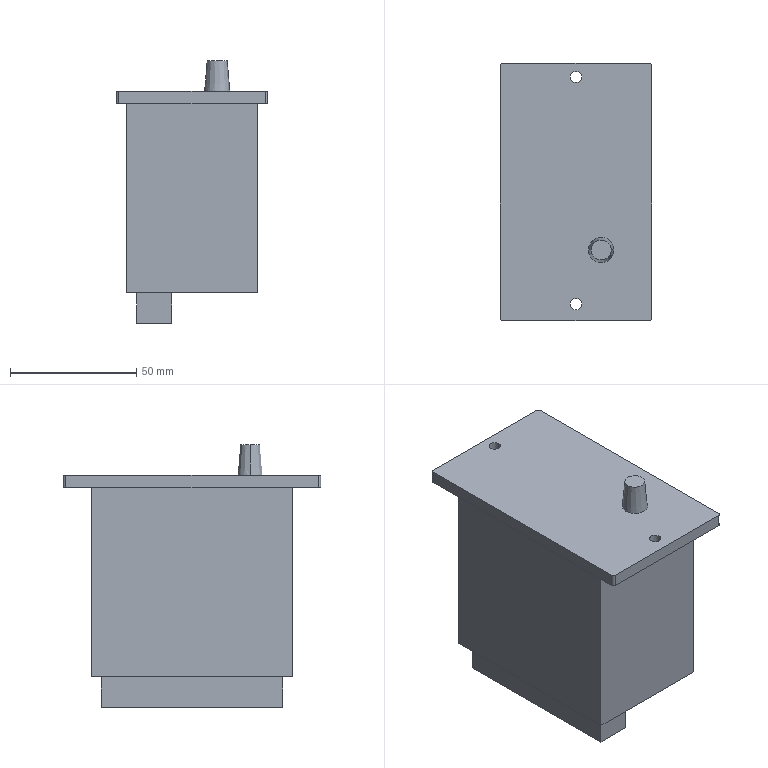Part | SolidWorks | features ICE 3, Extrusion 1, Fillet 1 | 1 solid | 27 faces | box 60 x 102 x 104 mm | volume 355291 mm3 | plane 17 | cylinder 8 | cone 2 | commonest cylinder face diameters 2 x4 4.5 x4
STEP:
#1=CARTESIAN_POINT('',(6.05,-23.,17.));
#2=VERTEX_POINT('',#1);
#3=CARTESIAN_POINT('',(13.95,-23.,17.));
#4=VERTEX_POINT('',#3);
#5=CARTESIAN_POINT('',(10.,-23.,17.));
#6=DIRECTION('',(0.,0.,1.));
#7=DIRECTION('',(1.,0.,0.));
#8=AXIS2_PLACEMENT_3D('',#5,#6,#7);
#9=CIRCLE('',#8,3.95);
#10=EDGE_CURVE('',#2,#4,#9,.T.);
#11=ORIENTED_EDGE('',*,*,#10,.F.);
#12=CARTESIAN_POINT('',(5.,-23.,5.));
#13=VERTEX_POINT('',#12);
#14=CARTESIAN_POINT('',(5.,-23.,5.));
#15=DIRECTION('',(-0.08716,0.,-0.9962));
#16=VECTOR('',#15,1000.);
#17=LINE('',#14,#16);
#18=EDGE_CURVE('',#2,#13,#17,.T.);
#19=ORIENTED_EDGE('',*,*,#18,.T.);
#20=CARTESIAN_POINT('',(15.,-23.,5.));
#21=VERTEX_POINT('',#20);
#22=CARTESIAN_POINT('',(10.,-23.,5.));
#23=DIRECTION('',(0.,0.,1.));
#24=DIRECTION('',(-1.,0.,0.));
#25=AXIS2_PLACEMENT_3D('',#22,#23,#24);
#26=CIRCLE('',#25,5.);
#27=EDGE_CURVE('',#13,#21,#26,.T.);
#28=ORIENTED_EDGE('',*,*,#27,.T.);
#29=CARTESIAN_POINT('',(15.,-23.,5.));
#30=DIRECTION('',(0.08716,0.,-0.9962));
#31=VECTOR('',#30,1000.);
#32=LINE('',#29,#31);
#33=EDGE_CURVE('',#4,#21,#32,.T.);
#34=ORIENTED_EDGE('',*,*,#33,.F.);
#35=EDGE_LOOP('',(#11,#19,#28,#34));
#36=FACE_OUTER_BOUND('',#35,.T.);
#37=CARTESIAN_POINT('',(10.,-23.,5.));
#38=DIRECTION('',(0.,0.,-1.));
#39=DIRECTION('',(1.,0.,0.));
#40=AXIS2_PLACEMENT_3D('',#37,#38,#39);
#41=CONICAL_SURFACE('',#40,5.,0.08727);
#42=ADVANCED_FACE('',(#36),#41,.T.);
#43=CARTESIAN_POINT('',(-2.25,-44.437,5.));
#44=VERTEX_POINT('',#43);
#45=CARTESIAN_POINT('',(2.25,-44.437,5.));
#46=VERTEX_POINT('',#45);
#47=CARTESIAN_POINT('',(0.,-44.437,5.));
#48=DIRECTION('',(0.,0.,1.));
#49=DIRECTION('',(1.,0.,0.));
#50=AXIS2_PLACEMENT_3D('',#47,#48,#49);
#51=CIRCLE('',#50,2.25);
#52=EDGE_CURVE('',#44,#46,#51,.T.);
#53=ORIENTED_EDGE('',*,*,#52,.T.);
#54=CARTESIAN_POINT('',(2.25,-44.437,0.));
#55=VERTEX_POINT('',#54);
#56=CARTESIAN_POINT('',(2.25,-44.437,5.));
#57=DIRECTION('',(0.,0.,-1.));
#58=VECTOR('',#57,1000.);
#59=LINE('',#56,#58);
#60=EDGE_CURVE('',#46,#55,#59,.T.);
#61=ORIENTED_EDGE('',*,*,#60,.T.);
#62=CARTESIAN_POINT('',(-2.25,-44.437,0.));
#63=VERTEX_POINT('',#62);
#64=CARTESIAN_POINT('',(0.,-44.437,0.));
#65=DIRECTION('',(0.,0.,1.));
#66=DIRECTION('',(1.,0.,0.));
#67=AXIS2_PLACEMENT_3D('',#64,#65,#66);
#68=CIRCLE('',#67,2.25);
#69=EDGE_CURVE('',#63,#55,#68,.T.);
#70=ORIENTED_EDGE('',*,*,#69,.F.);
#71=CARTESIAN_POINT('',(-2.25,-44.437,5.));
#72=DIRECTION('',(0.,0.,-1.));
#73=VECTOR('',#72,1000.);
#74=LINE('',#71,#73);
#75=EDGE_CURVE('',#44,#63,#74,.T.);
#76=ORIENTED_EDGE('',*,*,#75,.F.);
#77=EDGE_LOOP('',(#53,#61,#70,#76));
#78=FACE_OUTER_BOUND('',#77,.T.);
#79=CARTESIAN_POINT('',(0.,-44.437,5.));
#80=DIRECTION('',(0.,0.,-1.));
#81=DIRECTION('',(-1.,0.,0.));
#82=AXIS2_PLACEMENT_3D('',#79,#80,#81);
#83=CYLINDRICAL_SURFACE('',#82,2.25);
#84=ADVANCED_FACE('',(#78),#83,.F.);
#85=CARTESIAN_POINT('',(-2.25,45.563,5.));
#86=VERTEX_POINT('',#85);
#87=CARTESIAN_POINT('',(2.25,45.563,5.));
#88=VERTEX_POINT('',#87);
#89=CARTESIAN_POINT('',(0.,45.563,5.));
#90=DIRECTION('',(0.,0.,1.));
#91=DIRECTION('',(1.,0.,0.));
#92=AXIS2_PLACEMENT_3D('',#89,#90,#91);
#93=CIRCLE('',#92,2.25);
#94=EDGE_CURVE('',#86,#88,#93,.T.);
#95=ORIENTED_EDGE('',*,*,#94,.T.);
#96=CARTESIAN_POINT('',(2.25,45.563,0.));
#97=VERTEX_POINT('',#96);
#98=CARTESIAN_POINT('',(2.25,45.563,5.));
#99=DIRECTION('',(0.,0.,-1.));
#100=VECTOR('',#99,1000.);
#101=LINE('',#98,#100);
#102=EDGE_CURVE('',#88,#97,#101,.T.);
#103=ORIENTED_EDGE('',*,*,#102,.T.);
#104=CARTESIAN_POINT('',(-2.25,45.563,0.));
#105=VERTEX_POINT('',#104);
#106=CARTESIAN_POINT('',(0.,45.563,0.));
#107=DIRECTION('',(0.,0.,1.));
#108=DIRECTION('',(1.,0.,0.));
#109=AXIS2_PLACEMENT_3D('',#106,#107,#108);
#110=CIRCLE('',#109,2.25);
#111=EDGE_CURVE('',#105,#97,#110,.T.);
#112=ORIENTED_EDGE('',*,*,#111,.F.);
#113=CARTESIAN_POINT('',(-2.25,45.563,5.));
#114=DIRECTION('',(0.,0.,-1.));
#115=VECTOR('',#114,1000.);
#116=LINE('',#113,#115);
#117=EDGE_CURVE('',#86,#105,#116,.T.);
#118=ORIENTED_EDGE('',*,*,#117,.F.);
#119=EDGE_LOOP('',(#95,#103,#112,#118));
#120=FACE_OUTER_BOUND('',#119,.T.);
#121=CARTESIAN_POINT('',(0.,45.563,5.));
#122=DIRECTION('',(0.,0.,-1.));
#123=DIRECTION('',(-1.,0.,0.));
#124=AXIS2_PLACEMENT_3D('',#121,#122,#123);
#125=CYLINDRICAL_SURFACE('',#124,2.25);
#126=ADVANCED_FACE('',(#120),#125,.F.);
#127=CARTESIAN_POINT('',(-26.,-40.,-75.));
#128=VERTEX_POINT('',#127);
#129=CARTESIAN_POINT('',(-26.,40.,-75.));
#130=VERTEX_POINT('',#129);
#131=CARTESIAN_POINT('',(-26.,-40.,-75.));
#132=DIRECTION('',(0.,1.,0.));
#133=VECTOR('',#132,1000.);
#134=LINE('',#131,#133);
#135=EDGE_CURVE('',#128,#130,#134,.T.);
#136=ORIENTED_EDGE('',*,*,#135,.T.);
#137=CARTESIAN_POINT('',(26.,40.,-75.));
#138=VERTEX_POINT('',#137);
#139=CARTESIAN_POINT('',(26.,40.,-75.));
#140=DIRECTION('',(1.,0.,0.));
#141=VECTOR('',#140,1000.);
#142=LINE('',#139,#141);
#143=EDGE_CURVE('',#130,#138,#142,.T.);
#144=ORIENTED_EDGE('',*,*,#143,.T.);
#145=CARTESIAN_POINT('',(26.,-40.,-75.));
#146=VERTEX_POINT('',#145);
#147=CARTESIAN_POINT('',(26.,-40.,-75.));
#148=DIRECTION('',(0.,-1.,0.));
#149=VECTOR('',#148,1000.);
#150=LINE('',#147,#149);
#151=EDGE_CURVE('',#138,#146,#150,.T.);
#152=ORIENTED_EDGE('',*,*,#151,.T.);
#153=CARTESIAN_POINT('',(26.,-40.,-75.));
#154=DIRECTION('',(-1.,0.,0.));
#155=VECTOR('',#154,1000.);
#156=LINE('',#153,#155);
#157=EDGE_CURVE('',#146,#128,#156,.T.);
#158=ORIENTED_EDGE('',*,*,#157,.T.);
#159=EDGE_LOOP('',(#136,#144,#152,#158));
#160=FACE_OUTER_BOUND('',#159,.T.);
#161=CARTESIAN_POINT('',(-8.,36.,-75.));
#162=VERTEX_POINT('',#161);
#163=CARTESIAN_POINT('',(-8.,-36.,-75.));
#164=VERTEX_POINT('',#163);
#165=CARTESIAN_POINT('',(-8.,36.,-75.));
#166=DIRECTION('',(0.,-1.,0.));
#167=VECTOR('',#166,1000.);
#168=LINE('',#165,#167);
#169=EDGE_CURVE('',#162,#164,#168,.T.);
#170=ORIENTED_EDGE('',*,*,#169,.F.);
#171=CARTESIAN_POINT('',(-22.,36.,-75.));
#172=VERTEX_POINT('',#171);
#173=CARTESIAN_POINT('',(-8.,36.,-75.));
#174=DIRECTION('',(1.,0.,0.));
#175=VECTOR('',#174,1000.);
#176=LINE('',#173,#175);
#177=EDGE_CURVE('',#172,#162,#176,.T.);
#178=ORIENTED_EDGE('',*,*,#177,.F.);
#179=CARTESIAN_POINT('',(-22.,-36.,-75.));
#180=VERTEX_POINT('',#179);
#181=CARTESIAN_POINT('',(-22.,36.,-75.));
#182=DIRECTION('',(0.,1.,0.));
#183=VECTOR('',#182,1000.);
#184=LINE('',#181,#183);
#185=EDGE_CURVE('',#180,#172,#184,.T.);
#186=ORIENTED_EDGE('',*,*,#185,.F.);
#187=CARTESIAN_POINT('',(-8.,-36.,-75.));
#188=DIRECTION('',(-1.,0.,0.));
#189=VECTOR('',#188,1000.);
#190=LINE('',#187,#189);
#191=EDGE_CURVE('',#164,#180,#190,.T.);
#192=ORIENTED_EDGE('',*,*,#191,.F.);
#193=EDGE_LOOP('',(#170,#178,#186,#192));
#194=FACE_BOUND('',#193,.T.);
#195=CARTESIAN_POINT('',(0.,0.,-75.));
#196=DIRECTION('',(0.,0.,1.));
#197=DIRECTION('',(1.,0.,0.));
#198=AXIS2_PLACEMENT_3D('',#195,#196,#197);
#199=PLANE('',#198);
#200=ADVANCED_FACE('',(#160,#194),#199,.F.);
#201=ORIENTED_EDGE('',*,*,#52,.F.);
#202=CARTESIAN_POINT('',(0.,-44.437,5.));
#203=DIRECTION('',(0.,0.,1.));
#204=DIRECTION('',(1.,0.,0.));
#205=AXIS2_PLACEMENT_3D('',#202,#203,#204);
#206=CIRCLE('',#205,2.25);
#207=EDGE_CURVE('',#46,#44,#206,.T.);
#208=ORIENTED_EDGE('',*,*,#207,.F.);
#209=EDGE_LOOP('',(#201,#208));
#210=FACE_BOUND('',#209,.T.);
#211=CARTESIAN_POINT('',(-30.,50.,5.));
#212=VERTEX_POINT('',#211);
#213=CARTESIAN_POINT('',(-30.,-50.,5.));
#214=VERTEX_POINT('',#213);
#215=CARTESIAN_POINT('',(-30.,-51.,5.));
#216=DIRECTION('',(0.,-1.,0.));
#217=VECTOR('',#216,1000.);
#218=LINE('',#215,#217);
#219=EDGE_CURVE('',#212,#214,#218,.T.);
#220=ORIENTED_EDGE('',*,*,#219,.T.);
#221=CARTESIAN_POINT('',(-29.,-51.,5.));
#222=VERTEX_POINT('',#221);
#223=CARTESIAN_POINT('',(-29.,-50.,5.));
#224=DIRECTION('',(0.,0.,1.));
#225=DIRECTION('',(-1.,0.,0.));
#226=AXIS2_PLACEMENT_3D('',#223,#224,#225);
#227=CIRCLE('',#226,1.);
#228=EDGE_CURVE('',#214,#222,#227,.T.);
#229=ORIENTED_EDGE('',*,*,#228,.T.);
#230=CARTESIAN_POINT('',(29.,-51.,5.));
#231=VERTEX_POINT('',#230);
#232=CARTESIAN_POINT('',(-30.,-51.,5.));
#233=DIRECTION('',(1.,0.,0.));
#234=VECTOR('',#233,1000.);
#235=LINE('',#232,#234);
#236=EDGE_CURVE('',#222,#231,#235,.T.);
#237=ORIENTED_EDGE('',*,*,#236,.T.);
#238=CARTESIAN_POINT('',(30.,-50.,5.));
#239=VERTEX_POINT('',#238);
#240=CARTESIAN_POINT('',(29.,-50.,5.));
#241=DIRECTION('',(0.,0.,1.));
#242=DIRECTION('',(-1.,0.,0.));
#243=AXIS2_PLACEMENT_3D('',#240,#241,#242);
#244=CIRCLE('',#243,1.);
#245=EDGE_CURVE('',#231,#239,#244,.T.);
#246=ORIENTED_EDGE('',*,*,#245,.T.);
#247=CARTESIAN_POINT('',(30.,50.,5.));
#248=VERTEX_POINT('',#247);
#249=CARTESIAN_POINT('',(30.,-51.,5.));
#250=DIRECTION('',(0.,1.,0.));
#251=VECTOR('',#250,1000.);
#252=LINE('',#249,#251);
#253=EDGE_CURVE('',#239,#248,#252,.T.);
#254=ORIENTED_EDGE('',*,*,#253,.T.);
#255=CARTESIAN_POINT('',(29.,51.,5.));
#256=VERTEX_POINT('',#255);
#257=CARTESIAN_POINT('',(29.,50.,5.));
#258=DIRECTION('',(0.,0.,1.));
#259=DIRECTION('',(-1.,0.,0.));
#260=AXIS2_PLACEMENT_3D('',#257,#258,#259);
#261=CIRCLE('',#260,1.);
#262=EDGE_CURVE('',#248,#256,#261,.T.);
#263=ORIENTED_EDGE('',*,*,#262,.T.);
#264=CARTESIAN_POINT('',(-29.,51.,5.));
#265=VERTEX_POINT('',#264);
#266=CARTESIAN_POINT('',(-30.,51.,5.));
#267=DIRECTION('',(-1.,0.,0.));
#268=VECTOR('',#267,1000.);
#269=LINE('',#266,#268);
#270=EDGE_CURVE('',#256,#265,#269,.T.);
#271=ORIENTED_EDGE('',*,*,#270,.T.);
#272=CARTESIAN_POINT('',(-29.,50.,5.));
#273=DIRECTION('',(0.,0.,1.));
#274=DIRECTION('',(-1.,0.,0.));
#275=AXIS2_PLACEMENT_3D('',#272,#273,#274);
#276=CIRCLE('',#275,1.);
#277=EDGE_CURVE('',#265,#212,#276,.T.);
#278=ORIENTED_EDGE('',*,*,#277,.T.);
#279=EDGE_LOOP('',(#220,#229,#237,#246,#254,#263,#271,#278));
#280=FACE_OUTER_BOUND('',#279,.T.);
#281=ORIENTED_EDGE('',*,*,#94,.F.);
#282=CARTESIAN_POINT('',(0.,45.563,5.));
#283=DIRECTION('',(0.,0.,1.));
#284=DIRECTION('',(1.,0.,0.));
#285=AXIS2_PLACEMENT_3D('',#282,#283,#284);
#286=CIRCLE('',#285,2.25);
#287=EDGE_CURVE('',#88,#86,#286,.T.);
#288=ORIENTED_EDGE('',*,*,#287,.F.);
#289=EDGE_LOOP('',(#281,#288));
#290=FACE_BOUND('',#289,.T.);
#291=CARTESIAN_POINT('',(10.,-23.,5.));
#292=DIRECTION('',(0.,0.,1.));
#293=DIRECTION('',(-1.,0.,0.));
#294=AXIS2_PLACEMENT_3D('',#291,#292,#293);
#295=CIRCLE('',#294,5.);
#296=EDGE_CURVE('',#21,#13,#295,.T.);
#297=ORIENTED_EDGE('',*,*,#296,.F.);
#298=ORIENTED_EDGE('',*,*,#27,.F.);
#299=EDGE_LOOP('',(#297,#298));
#300=FACE_BOUND('',#299,.T.);
#301=CARTESIAN_POINT('',(0.,0.,5.));
#302=DIRECTION('',(0.,0.,-1.));
#303=DIRECTION('',(-1.,0.,0.));
#304=AXIS2_PLACEMENT_3D('',#301,#302,#303);
#305=PLANE('',#304);
#306=ADVANCED_FACE('',(#210,#280,#290,#300),#305,.F.);
#307=ORIENTED_EDGE('',*,*,#69,.T.);
#308=CARTESIAN_POINT('',(0.,-44.437,0.));
#309=DIRECTION('',(0.,0.,1.));
#310=DIRECTION('',(1.,0.,0.));
#311=AXIS2_PLACEMENT_3D('',#308,#309,#310);
#312=CIRCLE('',#311,2.25);
#313=EDGE_CURVE('',#55,#63,#312,.T.);
#314=ORIENTED_EDGE('',*,*,#313,.T.);
#315=EDGE_LOOP('',(#307,#314));
#316=FACE_BOUND('',#315,.T.);
#317=CARTESIAN_POINT('',(-29.,-51.,0.));
#318=VERTEX_POINT('',#317);
#319=CARTESIAN_POINT('',(29.,-51.,0.));
#320=VERTEX_POINT('',#319);
#321=CARTESIAN_POINT('',(-30.,-51.,0.));
#322=DIRECTION('',(1.,0.,0.));
#323=VECTOR('',#322,1000.);
#324=LINE('',#321,#323);
#325=EDGE_CURVE('',#318,#320,#324,.T.);
#326=ORIENTED_EDGE('',*,*,#325,.F.);
#327=CARTESIAN_POINT('',(-30.,-50.,0.));
#328=VERTEX_POINT('',#327);
#329=CARTESIAN_POINT('',(-29.,-50.,0.));
#330=DIRECTION('',(0.,0.,-1.));
#331=DIRECTION('',(-1.,0.,0.));
#332=AXIS2_PLACEMENT_3D('',#329,#330,#331);
#333=CIRCLE('',#332,1.);
#334=EDGE_CURVE('',#318,#328,#333,.T.);
#335=ORIENTED_EDGE('',*,*,#334,.T.);
#336=CARTESIAN_POINT('',(-30.,50.,0.));
#337=VERTEX_POINT('',#336);
#338=CARTESIAN_POINT('',(-30.,-51.,0.));
#339=DIRECTION('',(0.,-1.,0.));
#340=VECTOR('',#339,1000.);
#341=LINE('',#338,#340);
#342=EDGE_CURVE('',#337,#328,#341,.T.);
#343=ORIENTED_EDGE('',*,*,#342,.F.);
#344=CARTESIAN_POINT('',(-29.,51.,0.));
#345=VERTEX_POINT('',#344);
#346=CARTESIAN_POINT('',(-29.,50.,0.));
#347=DIRECTION('',(0.,0.,-1.));
#348=DIRECTION('',(-1.,0.,0.));
#349=AXIS2_PLACEMENT_3D('',#346,#347,#348);
#350=CIRCLE('',#349,1.);
#351=EDGE_CURVE('',#337,#345,#350,.T.);
#352=ORIENTED_EDGE('',*,*,#351,.T.);
#353=CARTESIAN_POINT('',(29.,51.,0.));
#354=VERTEX_POINT('',#353);
#355=CARTESIAN_POINT('',(-30.,51.,0.));
#356=DIRECTION('',(-1.,0.,0.));
#357=VECTOR('',#356,1000.);
#358=LINE('',#355,#357);
#359=EDGE_CURVE('',#354,#345,#358,.T.);
#360=ORIENTED_EDGE('',*,*,#359,.F.);
#361=CARTESIAN_POINT('',(30.,50.,0.));
#362=VERTEX_POINT('',#361);
#363=CARTESIAN_POINT('',(29.,50.,0.));
#364=DIRECTION('',(0.,0.,-1.));
#365=DIRECTION('',(-1.,0.,0.));
#366=AXIS2_PLACEMENT_3D('',#363,#364,#365);
#367=CIRCLE('',#366,1.);
#368=EDGE_CURVE('',#354,#362,#367,.T.);
#369=ORIENTED_EDGE('',*,*,#368,.T.);
#370=CARTESIAN_POINT('',(30.,-50.,0.));
#371=VERTEX_POINT('',#370);
#372=CARTESIAN_POINT('',(30.,-51.,0.));
#373=DIRECTION('',(0.,1.,0.));
#374=VECTOR('',#373,1000.);
#375=LINE('',#372,#374);
#376=EDGE_CURVE('',#371,#362,#375,.T.);
#377=ORIENTED_EDGE('',*,*,#376,.F.);
#378=CARTESIAN_POINT('',(29.,-50.,0.));
#379=DIRECTION('',(0.,0.,-1.));
#380=DIRECTION('',(-1.,0.,0.));
#381=AXIS2_PLACEMENT_3D('',#378,#379,#380);
#382=CIRCLE('',#381,1.);
#383=EDGE_CURVE('',#371,#320,#382,.T.);
#384=ORIENTED_EDGE('',*,*,#383,.T.);
#385=EDGE_LOOP('',(#326,#335,#343,#352,#360,#369,#377,#384));
#386=FACE_OUTER_BOUND('',#385,.T.);
#387=ORIENTED_EDGE('',*,*,#111,.T.);
#388=CARTESIAN_POINT('',(0.,45.563,0.));
#389=DIRECTION('',(0.,0.,1.));
#390=DIRECTION('',(1.,0.,0.));
#391=AXIS2_PLACEMENT_3D('',#388,#389,#390);
#392=CIRCLE('',#391,2.25);
#393=EDGE_CURVE('',#97,#105,#392,.T.);
#394=ORIENTED_EDGE('',*,*,#393,.T.);
#395=EDGE_LOOP('',(#387,#394));
#396=FACE_BOUND('',#395,.T.);
#397=CARTESIAN_POINT('',(-26.,40.,0.));
#398=VERTEX_POINT('',#397);
#399=CARTESIAN_POINT('',(26.,40.,0.));
#400=VERTEX_POINT('',#399);
#401=CARTESIAN_POINT('',(26.,40.,0.));
#402=DIRECTION('',(1.,0.,0.));
#403=VECTOR('',#402,1000.);
#404=LINE('',#401,#403);
#405=EDGE_CURVE('',#398,#400,#404,.T.);
#406=ORIENTED_EDGE('',*,*,#405,.F.);
#407=CARTESIAN_POINT('',(-26.,-40.,0.));
#408=VERTEX_POINT('',#407);
#409=CARTESIAN_POINT('',(-26.,-40.,0.));
#410=DIRECTION('',(0.,1.,0.));
#411=VECTOR('',#410,1000.);
#412=LINE('',#409,#411);
#413=EDGE_CURVE('',#408,#398,#412,.T.);
#414=ORIENTED_EDGE('',*,*,#413,.F.);
#415=CARTESIAN_POINT('',(26.,-40.,0.));
#416=VERTEX_POINT('',#415);
#417=CARTESIAN_POINT('',(26.,-40.,0.));
#418=DIRECTION('',(-1.,0.,0.));
#419=VECTOR('',#418,1000.);
#420=LINE('',#417,#419);
#421=EDGE_CURVE('',#416,#408,#420,.T.);
#422=ORIENTED_EDGE('',*,*,#421,.F.);
#423=CARTESIAN_POINT('',(26.,-40.,0.));
#424=DIRECTION('',(0.,-1.,0.));
#425=VECTOR('',#424,1000.);
#426=LINE('',#423,#425);
#427=EDGE_CURVE('',#400,#416,#426,.T.);
#428=ORIENTED_EDGE('',*,*,#427,.F.);
#429=EDGE_LOOP('',(#406,#414,#422,#428));
#430=FACE_BOUND('',#429,.T.);
#431=CARTESIAN_POINT('',(0.,0.,0.));
#432=DIRECTION('',(0.,0.,-1.));
#433=DIRECTION('',(-1.,0.,0.));
#434=AXIS2_PLACEMENT_3D('',#431,#432,#433);
#435=PLANE('',#434);
#436=ADVANCED_FACE('',(#316,#386,#396,#430),#435,.T.);
#437=ORIENTED_EDGE('',*,*,#253,.F.);
#438=CARTESIAN_POINT('',(30.,-50.,5.));
#439=DIRECTION('',(0.,0.,-1.));
#440=VECTOR('',#439,1000.);
#441=LINE('',#438,#440);
#442=EDGE_CURVE('',#239,#371,#441,.T.);
#443=ORIENTED_EDGE('',*,*,#442,.T.);
#444=ORIENTED_EDGE('',*,*,#376,.T.);
#445=CARTESIAN_POINT('',(30.,50.,5.));
#446=DIRECTION('',(0.,0.,1.));
#447=VECTOR('',#446,1000.);
#448=LINE('',#445,#447);
#449=EDGE_CURVE('',#362,#248,#448,.T.);
#450=ORIENTED_EDGE('',*,*,#449,.T.);
#451=EDGE_LOOP('',(#437,#443,#444,#450));
#452=FACE_OUTER_BOUND('',#451,.T.);
#453=CARTESIAN_POINT('',(30.,-51.,5.));
#454=DIRECTION('',(-1.,0.,0.));
#455=DIRECTION('',(0.,0.,1.));
#456=AXIS2_PLACEMENT_3D('',#453,#454,#455);
#457=PLANE('',#456);
#458=ADVANCED_FACE('',(#452),#457,.F.);
#459=ORIENTED_EDGE('',*,*,#270,.F.);
#460=CARTESIAN_POINT('',(29.,51.,5.));
#461=DIRECTION('',(0.,0.,-1.));
#462=VECTOR('',#461,1000.);
#463=LINE('',#460,#462);
#464=EDGE_CURVE('',#256,#354,#463,.T.);
#465=ORIENTED_EDGE('',*,*,#464,.T.);
#466=ORIENTED_EDGE('',*,*,#359,.T.);
#467=CARTESIAN_POINT('',(-29.,51.,5.));
#468=DIRECTION('',(0.,0.,1.));
#469=VECTOR('',#468,1000.);
#470=LINE('',#467,#469);
#471=EDGE_CURVE('',#345,#265,#470,.T.);
#472=ORIENTED_EDGE('',*,*,#471,.T.);
#473=EDGE_LOOP('',(#459,#465,#466,#472));
#474=FACE_OUTER_BOUND('',#473,.T.);
#475=CARTESIAN_POINT('',(-30.,51.,5.));
#476=DIRECTION('',(0.,-1.,0.));
#477=DIRECTION('',(0.,0.,-1.));
#478=AXIS2_PLACEMENT_3D('',#475,#476,#477);
#479=PLANE('',#478);
#480=ADVANCED_FACE('',(#474),#479,.F.);
#481=ORIENTED_EDGE('',*,*,#342,.T.);
#482=CARTESIAN_POINT('',(-30.,-50.,5.));
#483=DIRECTION('',(0.,0.,1.));
#484=VECTOR('',#483,1000.);
#485=LINE('',#482,#484);
#486=EDGE_CURVE('',#328,#214,#485,.T.);
#487=ORIENTED_EDGE('',*,*,#486,.T.);
#488=ORIENTED_EDGE('',*,*,#219,.F.);
#489=CARTESIAN_POINT('',(-30.,50.,5.));
#490=DIRECTION('',(0.,0.,-1.));
#491=VECTOR('',#490,1000.);
#492=LINE('',#489,#491);
#493=EDGE_CURVE('',#212,#337,#492,.T.);
#494=ORIENTED_EDGE('',*,*,#493,.T.);
#495=EDGE_LOOP('',(#481,#487,#488,#494));
#496=FACE_OUTER_BOUND('',#495,.T.);
#497=CARTESIAN_POINT('',(-30.,-51.,5.));
#498=DIRECTION('',(1.,0.,0.));
#499=DIRECTION('',(0.,0.,-1.));
#500=AXIS2_PLACEMENT_3D('',#497,#498,#499);
#501=PLANE('',#500);
#502=ADVANCED_FACE('',(#496),#501,.F.);
#503=ORIENTED_EDGE('',*,*,#236,.F.);
#504=CARTESIAN_POINT('',(-29.,-51.,5.));
#505=DIRECTION('',(0.,0.,-1.));
#506=VECTOR('',#505,1000.);
#507=LINE('',#504,#506);
#508=EDGE_CURVE('',#222,#318,#507,.T.);
#509=ORIENTED_EDGE('',*,*,#508,.T.);
#510=ORIENTED_EDGE('',*,*,#325,.T.);
#511=CARTESIAN_POINT('',(29.,-51.,5.));
#512=DIRECTION('',(0.,0.,1.));
#513=VECTOR('',#512,1000.);
#514=LINE('',#511,#513);
#515=EDGE_CURVE('',#320,#231,#514,.T.);
#516=ORIENTED_EDGE('',*,*,#515,.T.);
#517=EDGE_LOOP('',(#503,#509,#510,#516));
#518=FACE_OUTER_BOUND('',#517,.T.);
#519=CARTESIAN_POINT('',(-30.,-51.,5.));
#520=DIRECTION('',(0.,1.,0.));
#521=DIRECTION('',(0.,0.,1.));
#522=AXIS2_PLACEMENT_3D('',#519,#520,#521);
#523=PLANE('',#522);
#524=ADVANCED_FACE('',(#518),#523,.F.);
#525=ORIENTED_EDGE('',*,*,#102,.F.);
#526=ORIENTED_EDGE('',*,*,#287,.T.);
#527=ORIENTED_EDGE('',*,*,#117,.T.);
#528=ORIENTED_EDGE('',*,*,#393,.F.);
#529=EDGE_LOOP('',(#525,#526,#527,#528));
#530=FACE_OUTER_BOUND('',#529,.T.);
#531=CARTESIAN_POINT('',(0.,45.563,5.));
#532=DIRECTION('',(0.,0.,-1.));
#533=DIRECTION('',(-1.,0.,0.));
#534=AXIS2_PLACEMENT_3D('',#531,#532,#533);
#535=CYLINDRICAL_SURFACE('',#534,2.25);
#536=ADVANCED_FACE('',(#530),#535,.F.);
#537=ORIENTED_EDGE('',*,*,#60,.F.);
#538=ORIENTED_EDGE('',*,*,#207,.T.);
#539=ORIENTED_EDGE('',*,*,#75,.T.);
#540=ORIENTED_EDGE('',*,*,#313,.F.);
#541=EDGE_LOOP('',(#537,#538,#539,#540));
#542=FACE_OUTER_BOUND('',#541,.T.);
#543=CARTESIAN_POINT('',(0.,-44.437,5.));
#544=DIRECTION('',(0.,0.,-1.));
#545=DIRECTION('',(-1.,0.,0.));
#546=AXIS2_PLACEMENT_3D('',#543,#544,#545);
#547=CYLINDRICAL_SURFACE('',#546,2.25);
#548=ADVANCED_FACE('',(#542),#547,.F.);
#549=ORIENTED_EDGE('',*,*,#413,.T.);
#550=CARTESIAN_POINT('',(-26.,40.,-75.));
#551=DIRECTION('',(0.,0.,1.));
#552=VECTOR('',#551,1000.);
#553=LINE('',#550,#552);
#554=EDGE_CURVE('',#130,#398,#553,.T.);
#555=ORIENTED_EDGE('',*,*,#554,.F.);
#556=ORIENTED_EDGE('',*,*,#135,.F.);
#557=CARTESIAN_POINT('',(-26.,-40.,-75.));
#558=DIRECTION('',(0.,0.,1.));
#559=VECTOR('',#558,1000.);
#560=LINE('',#557,#559);
#561=EDGE_CURVE('',#128,#408,#560,.T.);
#562=ORIENTED_EDGE('',*,*,#561,.T.);
#563=EDGE_LOOP('',(#549,#555,#556,#562));
#564=FACE_OUTER_BOUND('',#563,.T.);
#565=CARTESIAN_POINT('',(-26.,-40.,-75.));
#566=DIRECTION('',(1.,0.,0.));
#567=DIRECTION('',(0.,0.,-1.));
#568=AXIS2_PLACEMENT_3D('',#565,#566,#567);
#569=PLANE('',#568);
#570=ADVANCED_FACE('',(#564),#569,.F.);
#571=ORIENTED_EDGE('',*,*,#405,.T.);
#572=CARTESIAN_POINT('',(26.,40.,-75.));
#573=DIRECTION('',(0.,0.,1.));
#574=VECTOR('',#573,1000.);
#575=LINE('',#572,#574);
#576=EDGE_CURVE('',#138,#400,#575,.T.);
#577=ORIENTED_EDGE('',*,*,#576,.F.);
#578=ORIENTED_EDGE('',*,*,#143,.F.);
#579=ORIENTED_EDGE('',*,*,#554,.T.);
#580=EDGE_LOOP('',(#571,#577,#578,#579));
#581=FACE_OUTER_BOUND('',#580,.T.);
#582=CARTESIAN_POINT('',(26.,40.,-75.));
#583=DIRECTION('',(0.,-1.,0.));
#584=DIRECTION('',(0.,0.,-1.));
#585=AXIS2_PLACEMENT_3D('',#582,#583,#584);
#586=PLANE('',#585);
#587=ADVANCED_FACE('',(#581),#586,.F.);
#588=ORIENTED_EDGE('',*,*,#427,.T.);
#589=CARTESIAN_POINT('',(26.,-40.,-75.));
#590=DIRECTION('',(0.,0.,1.));
#591=VECTOR('',#590,1000.);
#592=LINE('',#589,#591);
#593=EDGE_CURVE('',#146,#416,#592,.T.);
#594=ORIENTED_EDGE('',*,*,#593,.F.);
#595=ORIENTED_EDGE('',*,*,#151,.F.);
#596=ORIENTED_EDGE('',*,*,#576,.T.);
#597=EDGE_LOOP('',(#588,#594,#595,#596));
#598=FACE_OUTER_BOUND('',#597,.T.);
#599=CARTESIAN_POINT('',(26.,-40.,-75.));
#600=DIRECTION('',(-1.,0.,0.));
#601=DIRECTION('',(0.,0.,1.));
#602=AXIS2_PLACEMENT_3D('',#599,#600,#601);
#603=PLANE('',#602);
#604=ADVANCED_FACE('',(#598),#603,.F.);
#605=ORIENTED_EDGE('',*,*,#421,.T.);
#606=ORIENTED_EDGE('',*,*,#561,.F.);
#607=ORIENTED_EDGE('',*,*,#157,.F.);
#608=ORIENTED_EDGE('',*,*,#593,.T.);
#609=EDGE_LOOP('',(#605,#606,#607,#608));
#610=FACE_OUTER_BOUND('',#609,.T.);
#611=CARTESIAN_POINT('',(26.,-40.,-75.));
#612=DIRECTION('',(0.,1.,0.));
#613=DIRECTION('',(0.,0.,1.));
#614=AXIS2_PLACEMENT_3D('',#611,#612,#613);
#615=PLANE('',#614);
#616=ADVANCED_FACE('',(#610),#615,.F.);
#617=ORIENTED_EDGE('',*,*,#18,.F.);
#618=CARTESIAN_POINT('',(10.,-23.,17.));
#619=DIRECTION('',(0.,0.,1.));
#620=DIRECTION('',(1.,0.,0.));
#621=AXIS2_PLACEMENT_3D('',#618,#619,#620);
#622=CIRCLE('',#621,3.95);
#623=EDGE_CURVE('',#4,#2,#622,.T.);
#624=ORIENTED_EDGE('',*,*,#623,.F.);
#625=ORIENTED_EDGE('',*,*,#33,.T.);
#626=ORIENTED_EDGE('',*,*,#296,.T.);
#627=EDGE_LOOP('',(#617,#624,#625,#626));
#628=FACE_OUTER_BOUND('',#627,.T.);
#629=CARTESIAN_POINT('',(10.,-23.,5.));
#630=DIRECTION('',(0.,0.,-1.));
#631=DIRECTION('',(1.,0.,0.));
#632=AXIS2_PLACEMENT_3D('',#629,#630,#631);
#633=CONICAL_SURFACE('',#632,5.,0.08727);
#634=ADVANCED_FACE('',(#628),#633,.T.);
#635=ORIENTED_EDGE('',*,*,#623,.T.);
#636=ORIENTED_EDGE('',*,*,#10,.T.);
#637=EDGE_LOOP('',(#635,#636));
#638=FACE_OUTER_BOUND('',#637,.T.);
#639=CARTESIAN_POINT('',(10.,-23.,17.));
#640=DIRECTION('',(0.,0.,1.));
#641=DIRECTION('',(1.,0.,0.));
#642=AXIS2_PLACEMENT_3D('',#639,#640,#641);
#643=PLANE('',#642);
#644=ADVANCED_FACE('',(#638),#643,.T.);
#645=ORIENTED_EDGE('',*,*,#228,.F.);
#646=ORIENTED_EDGE('',*,*,#486,.F.);
#647=ORIENTED_EDGE('',*,*,#334,.F.);
#648=ORIENTED_EDGE('',*,*,#508,.F.);
#649=EDGE_LOOP('',(#645,#646,#647,#648));
#650=FACE_OUTER_BOUND('',#649,.T.);
#651=CARTESIAN_POINT('',(-29.,-50.,5.));
#652=DIRECTION('',(0.,0.,-1.));
#653=DIRECTION('',(-1.,0.,0.));
#654=AXIS2_PLACEMENT_3D('',#651,#652,#653);
#655=CYLINDRICAL_SURFACE('',#654,1.);
#656=ADVANCED_FACE('',(#650),#655,.T.);
#657=ORIENTED_EDGE('',*,*,#245,.F.);
#658=ORIENTED_EDGE('',*,*,#515,.F.);
#659=ORIENTED_EDGE('',*,*,#383,.F.);
#660=ORIENTED_EDGE('',*,*,#442,.F.);
#661=EDGE_LOOP('',(#657,#658,#659,#660));
#662=FACE_OUTER_BOUND('',#661,.T.);
#663=CARTESIAN_POINT('',(29.,-50.,5.));
#664=DIRECTION('',(0.,0.,-1.));
#665=DIRECTION('',(-1.,0.,0.));
#666=AXIS2_PLACEMENT_3D('',#663,#664,#665);
#667=CYLINDRICAL_SURFACE('',#666,1.);
#668=ADVANCED_FACE('',(#662),#667,.T.);
#669=ORIENTED_EDGE('',*,*,#262,.F.);
#670=ORIENTED_EDGE('',*,*,#449,.F.);
#671=ORIENTED_EDGE('',*,*,#368,.F.);
#672=ORIENTED_EDGE('',*,*,#464,.F.);
#673=EDGE_LOOP('',(#669,#670,#671,#672));
#674=FACE_OUTER_BOUND('',#673,.T.);
#675=CARTESIAN_POINT('',(29.,50.,5.));
#676=DIRECTION('',(0.,0.,-1.));
#677=DIRECTION('',(-1.,0.,0.));
#678=AXIS2_PLACEMENT_3D('',#675,#676,#677);
#679=CYLINDRICAL_SURFACE('',#678,1.);
#680=ADVANCED_FACE('',(#674),#679,.T.);
#681=ORIENTED_EDGE('',*,*,#277,.F.);
#682=ORIENTED_EDGE('',*,*,#471,.F.);
#683=ORIENTED_EDGE('',*,*,#351,.F.);
#684=ORIENTED_EDGE('',*,*,#493,.F.);
#685=EDGE_LOOP('',(#681,#682,#683,#684));
#686=FACE_OUTER_BOUND('',#685,.T.);
#687=CARTESIAN_POINT('',(-29.,50.,5.));
#688=DIRECTION('',(0.,0.,-1.));
#689=DIRECTION('',(-1.,0.,0.));
#690=AXIS2_PLACEMENT_3D('',#687,#688,#689);
#691=CYLINDRICAL_SURFACE('',#690,1.);
#692=ADVANCED_FACE('',(#686),#691,.T.);
#693=ORIENTED_EDGE('',*,*,#169,.T.);
#694=CARTESIAN_POINT('',(-8.,-36.,-87.));
#695=VERTEX_POINT('',#694);
#696=CARTESIAN_POINT('',(-8.,-36.,-87.));
#697=DIRECTION('',(0.,0.,1.));
#698=VECTOR('',#697,1000.);
#699=LINE('',#696,#698);
#700=EDGE_CURVE('',#695,#164,#699,.T.);
#701=ORIENTED_EDGE('',*,*,#700,.F.);
#702=CARTESIAN_POINT('',(-8.,36.,-87.));
#703=VERTEX_POINT('',#702);
#704=CARTESIAN_POINT('',(-8.,36.,-87.));
#705=DIRECTION('',(0.,-1.,0.));
#706=VECTOR('',#705,1000.);
#707=LINE('',#704,#706);
#708=EDGE_CURVE('',#703,#695,#707,.T.);
#709=ORIENTED_EDGE('',*,*,#708,.F.);
#710=CARTESIAN_POINT('',(-8.,36.,-87.));
#711=DIRECTION('',(0.,0.,1.));
#712=VECTOR('',#711,1000.);
#713=LINE('',#710,#712);
#714=EDGE_CURVE('',#703,#162,#713,.T.);
#715=ORIENTED_EDGE('',*,*,#714,.T.);
#716=EDGE_LOOP('',(#693,#701,#709,#715));
#717=FACE_OUTER_BOUND('',#716,.T.);
#718=CARTESIAN_POINT('',(-8.,36.,-87.));
#719=DIRECTION('',(-1.,0.,0.));
#720=DIRECTION('',(0.,-1.,0.));
#721=AXIS2_PLACEMENT_3D('',#718,#719,#720);
#722=PLANE('',#721);
#723=ADVANCED_FACE('',(#717),#722,.F.);
#724=ORIENTED_EDGE('',*,*,#191,.T.);
#725=CARTESIAN_POINT('',(-22.,-36.,-87.));
#726=VERTEX_POINT('',#725);
#727=CARTESIAN_POINT('',(-22.,-36.,-87.));
#728=DIRECTION('',(0.,0.,1.));
#729=VECTOR('',#728,1000.);
#730=LINE('',#727,#729);
#731=EDGE_CURVE('',#726,#180,#730,.T.);
#732=ORIENTED_EDGE('',*,*,#731,.F.);
#733=CARTESIAN_POINT('',(-8.,-36.,-87.));
#734=DIRECTION('',(-1.,0.,0.));
#735=VECTOR('',#734,1000.);
#736=LINE('',#733,#735);
#737=EDGE_CURVE('',#695,#726,#736,.T.);
#738=ORIENTED_EDGE('',*,*,#737,.F.);
#739=ORIENTED_EDGE('',*,*,#700,.T.);
#740=EDGE_LOOP('',(#724,#732,#738,#739));
#741=FACE_OUTER_BOUND('',#740,.T.);
#742=CARTESIAN_POINT('',(-8.,-36.,-87.));
#743=DIRECTION('',(0.,1.,0.));
#744=DIRECTION('',(0.,0.,1.));
#745=AXIS2_PLACEMENT_3D('',#742,#743,#744);
#746=PLANE('',#745);
#747=ADVANCED_FACE('',(#741),#746,.F.);
#748=ORIENTED_EDGE('',*,*,#185,.T.);
#749=CARTESIAN_POINT('',(-22.,36.,-87.));
#750=VERTEX_POINT('',#749);
#751=CARTESIAN_POINT('',(-22.,36.,-87.));
#752=DIRECTION('',(0.,0.,1.));
#753=VECTOR('',#752,1000.);
#754=LINE('',#751,#753);
#755=EDGE_CURVE('',#750,#172,#754,.T.);
#756=ORIENTED_EDGE('',*,*,#755,.F.);
#757=CARTESIAN_POINT('',(-22.,36.,-87.));
#758=DIRECTION('',(0.,1.,0.));
#759=VECTOR('',#758,1000.);
#760=LINE('',#757,#759);
#761=EDGE_CURVE('',#726,#750,#760,.T.);
#762=ORIENTED_EDGE('',*,*,#761,.F.);
#763=ORIENTED_EDGE('',*,*,#731,.T.);
#764=EDGE_LOOP('',(#748,#756,#762,#763));
#765=FACE_OUTER_BOUND('',#764,.T.);
#766=CARTESIAN_POINT('',(-22.,36.,-87.));
#767=DIRECTION('',(1.,0.,0.));
#768=DIRECTION('',(0.,1.,0.));
#769=AXIS2_PLACEMENT_3D('',#766,#767,#768);
#770=PLANE('',#769);
#771=ADVANCED_FACE('',(#765),#770,.F.);
#772=ORIENTED_EDGE('',*,*,#177,.T.);
#773=ORIENTED_EDGE('',*,*,#714,.F.);
#774=CARTESIAN_POINT('',(-8.,36.,-87.));
#775=DIRECTION('',(1.,0.,0.));
#776=VECTOR('',#775,1000.);
#777=LINE('',#774,#776);
#778=EDGE_CURVE('',#750,#703,#777,.T.);
#779=ORIENTED_EDGE('',*,*,#778,.F.);
#780=ORIENTED_EDGE('',*,*,#755,.T.);
#781=EDGE_LOOP('',(#772,#773,#779,#780));
#782=FACE_OUTER_BOUND('',#781,.T.);
#783=CARTESIAN_POINT('',(-8.,36.,-87.));
#784=DIRECTION('',(0.,-1.,0.));
#785=DIRECTION('',(0.,0.,-1.));
#786=AXIS2_PLACEMENT_3D('',#783,#784,#785);
#787=PLANE('',#786);
#788=ADVANCED_FACE('',(#782),#787,.F.);
#789=ORIENTED_EDGE('',*,*,#708,.T.);
#790=ORIENTED_EDGE('',*,*,#737,.T.);
#791=ORIENTED_EDGE('',*,*,#761,.T.);
#792=ORIENTED_EDGE('',*,*,#778,.T.);
#793=EDGE_LOOP('',(#789,#790,#791,#792));
#794=FACE_OUTER_BOUND('',#793,.T.);
#795=CARTESIAN_POINT('',(0.,0.,-87.));
#796=DIRECTION('',(0.,0.,-1.));
#797=DIRECTION('',(-1.,0.,0.));
#798=AXIS2_PLACEMENT_3D('',#795,#796,#797);
#799=PLANE('',#798);
#800=ADVANCED_FACE('',(#794),#799,.T.);
#801=CLOSED_SHELL('',(#42,#84,#126,#200,#306,#436,#458,#480,#502,#524,#536,#548,#570,#587,#604,#616,#634,#644,#656,#668,#680,#692,#723,#747,#771,#788,#800));
#802=MANIFOLD_SOLID_BREP('',#801);
#803=CARTESIAN_POINT('',(0.,0.,0.));
#804=DIRECTION('',(0.,0.,1.));
#805=DIRECTION('',(1.,0.,0.));
#806=AXIS2_PLACEMENT_3D('',#803,#804,#805);
#807=(LENGTH_UNIT()NAMED_UNIT(*)SI_UNIT(.MILLI.,.METRE.));
#808=UNCERTAINTY_MEASURE_WITH_UNIT(LENGTH_MEASURE(0.00001),#807,'','');
#809=(NAMED_UNIT(*)PLANE_ANGLE_UNIT()SI_UNIT($,.RADIAN.));
#810=(NAMED_UNIT(*)SI_UNIT($,.STERADIAN.)SOLID_ANGLE_UNIT());
#811=(GEOMETRIC_REPRESENTATION_CONTEXT(3)GLOBAL_UNCERTAINTY_ASSIGNED_CONTEXT((#808))GLOBAL_UNIT_ASSIGNED_CONTEXT((#807,#809,#810))REPRESENTATION_CONTEXT('',''));
#812=ADVANCED_BREP_SHAPE_REPRESENTATION('',(#802,#806),#811);